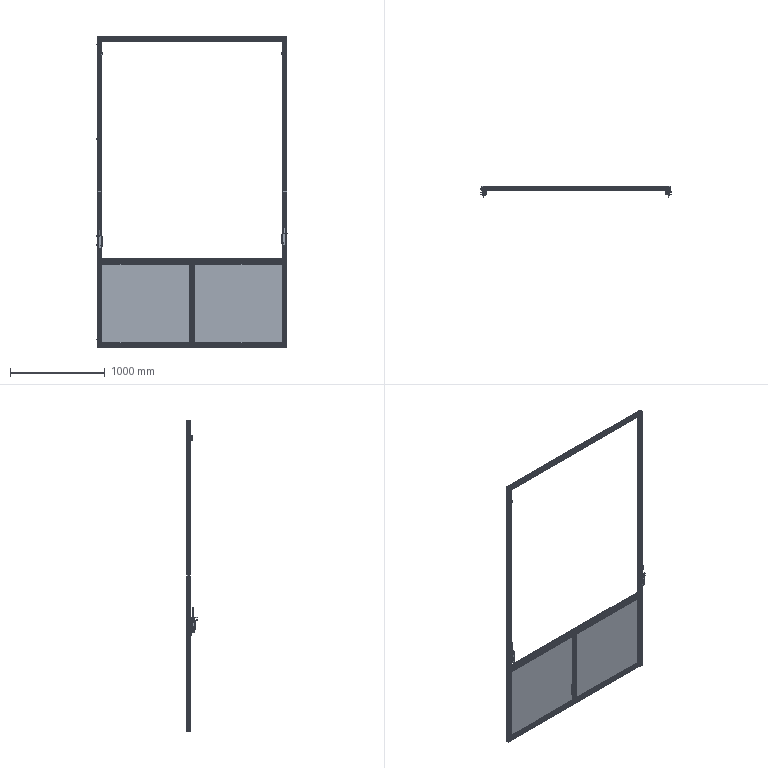Part | SolidWorks | features ReferencePattern 19, LocalLPattern 3, DerivedHolePattern 2 | 149 solids | 11540 faces | volume 17564416 mm3 | plane 6392 | cylinder 3030 | cone 1324 | spline 454 | torus 272 | sphere 68 | commonest cylinder face diameters 2.5 x336 1 x280 2 x248 0.562 x160 0.4 x148 8 x116